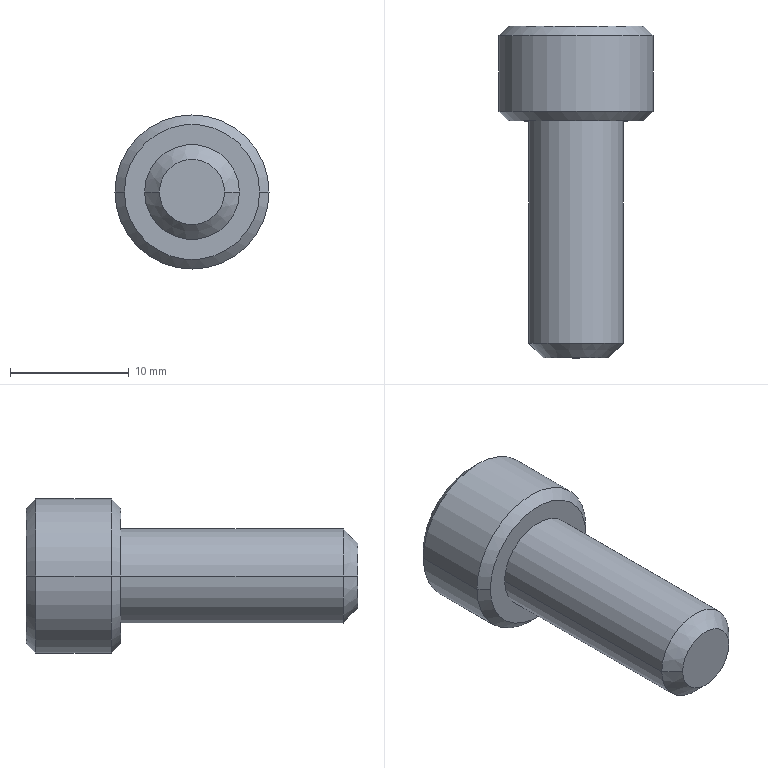Part | STEP file | BB62-M8-20L-1 | 1 solid | 27 faces | box 13 x 28 x 13 mm | volume 1878 mm3 | plane 15 | cone 8 | cylinder 4 | commonest cylinder face diameters 8 x2 13 x2
STEP:
#1=CARTESIAN_POINT('',(0.,2.02,0.));
#2=VERTEX_POINT('',#1);
#3=CARTESIAN_POINT('',(3.43,4.,0.));
#4=VERTEX_POINT('',#3);
#5=CARTESIAN_POINT('',(0.,2.02,0.));
#6=DIRECTION('',(0.866,0.5,0.));
#7=VECTOR('',#6,1000.);
#8=LINE('',#5,#7);
#9=EDGE_CURVE('',#2,#4,#8,.T.);
#10=ORIENTED_EDGE('',*,*,#9,.F.);
#11=CARTESIAN_POINT('',(-3.43,4.,0.));
#12=VERTEX_POINT('',#11);
#13=CARTESIAN_POINT('',(0.,2.02,0.));
#14=DIRECTION('',(-0.866,0.5,0.));
#15=VECTOR('',#14,1000.);
#16=LINE('',#13,#15);
#17=EDGE_CURVE('',#2,#12,#16,.T.);
#18=ORIENTED_EDGE('',*,*,#17,.T.);
#19=CARTESIAN_POINT('',(-2.97,4.,1.715));
#20=VERTEX_POINT('',#19);
#21=CARTESIAN_POINT('',(0.,4.,0.));
#22=DIRECTION('',(0.,-1.,0.));
#23=DIRECTION('',(-1.,0.,0.));
#24=AXIS2_PLACEMENT_3D('',#21,#22,#23);
#25=CIRCLE('',#24,3.43);
#26=EDGE_CURVE('',#20,#12,#25,.T.);
#27=ORIENTED_EDGE('',*,*,#26,.F.);
#28=CARTESIAN_POINT('',(0.,4.,3.43));
#29=VERTEX_POINT('',#28);
#30=CARTESIAN_POINT('',(0.,4.,0.));
#31=DIRECTION('',(0.,-1.,0.));
#32=DIRECTION('',(-1.,0.,0.));
#33=AXIS2_PLACEMENT_3D('',#30,#31,#32);
#34=CIRCLE('',#33,3.43);
#35=EDGE_CURVE('',#29,#20,#34,.T.);
#36=ORIENTED_EDGE('',*,*,#35,.F.);
#37=CARTESIAN_POINT('',(2.97,4.,1.715));
#38=VERTEX_POINT('',#37);
#39=CARTESIAN_POINT('',(0.,4.,0.));
#40=DIRECTION('',(0.,-1.,0.));
#41=DIRECTION('',(-1.,0.,0.));
#42=AXIS2_PLACEMENT_3D('',#39,#40,#41);
#43=CIRCLE('',#42,3.43);
#44=EDGE_CURVE('',#38,#29,#43,.T.);
#45=ORIENTED_EDGE('',*,*,#44,.F.);
#46=CARTESIAN_POINT('',(0.,4.,0.));
#47=DIRECTION('',(0.,-1.,0.));
#48=DIRECTION('',(-1.,0.,0.));
#49=AXIS2_PLACEMENT_3D('',#46,#47,#48);
#50=CIRCLE('',#49,3.43);
#51=EDGE_CURVE('',#4,#38,#50,.T.);
#52=ORIENTED_EDGE('',*,*,#51,.F.);
#53=EDGE_LOOP('',(#10,#18,#27,#36,#45,#52));
#54=FACE_OUTER_BOUND('',#53,.T.);
#55=CARTESIAN_POINT('',(0.,1002.02,0.));
#56=DIRECTION('',(0.,1.,0.));
#57=DIRECTION('',(1.,0.,0.));
#58=AXIS2_PLACEMENT_3D('',#55,#56,#57);
#59=CONICAL_SURFACE('',#58,1732.051,1.047);
#60=ADVANCED_FACE('',(#54),#59,.F.);
#61=CARTESIAN_POINT('',(2.75,-20.,0.));
#62=VERTEX_POINT('',#61);
#63=CARTESIAN_POINT('',(-2.75,-20.,0.));
#64=VERTEX_POINT('',#63);
#65=CARTESIAN_POINT('',(0.,-20.,0.));
#66=DIRECTION('',(0.,1.,0.));
#67=DIRECTION('',(1.,0.,0.));
#68=AXIS2_PLACEMENT_3D('',#65,#66,#67);
#69=CIRCLE('',#68,2.75);
#70=EDGE_CURVE('',#62,#64,#69,.T.);
#71=ORIENTED_EDGE('',*,*,#70,.T.);
#72=CARTESIAN_POINT('',(-4.,-18.75,0.));
#73=VERTEX_POINT('',#72);
#74=CARTESIAN_POINT('',(-2.75,-20.,0.));
#75=DIRECTION('',(-0.7071,0.7071,0.));
#76=VECTOR('',#75,1000.);
#77=LINE('',#74,#76);
#78=EDGE_CURVE('',#64,#73,#77,.T.);
#79=ORIENTED_EDGE('',*,*,#78,.T.);
#80=CARTESIAN_POINT('',(4.,-18.75,0.));
#81=VERTEX_POINT('',#80);
#82=CARTESIAN_POINT('',(0.,-18.75,0.));
#83=DIRECTION('',(0.,-1.,0.));
#84=DIRECTION('',(-1.,0.,0.));
#85=AXIS2_PLACEMENT_3D('',#82,#83,#84);
#86=CIRCLE('',#85,4.);
#87=EDGE_CURVE('',#73,#81,#86,.T.);
#88=ORIENTED_EDGE('',*,*,#87,.T.);
#89=CARTESIAN_POINT('',(2.75,-20.,0.));
#90=DIRECTION('',(0.7071,0.7071,0.));
#91=VECTOR('',#90,1000.);
#92=LINE('',#89,#91);
#93=EDGE_CURVE('',#62,#81,#92,.T.);
#94=ORIENTED_EDGE('',*,*,#93,.F.);
#95=EDGE_LOOP('',(#71,#79,#88,#94));
#96=FACE_OUTER_BOUND('',#95,.T.);
#97=CARTESIAN_POINT('',(0.,-20.,0.));
#98=DIRECTION('',(0.,1.,0.));
#99=DIRECTION('',(1.,0.,0.));
#100=AXIS2_PLACEMENT_3D('',#97,#98,#99);
#101=CONICAL_SURFACE('',#100,2.75,0.7854);
#102=ADVANCED_FACE('',(#96),#101,.T.);
#103=ORIENTED_EDGE('',*,*,#87,.F.);
#104=CARTESIAN_POINT('',(-4.,0.,0.));
#105=VERTEX_POINT('',#104);
#106=CARTESIAN_POINT('',(-4.,-18.75,0.));
#107=DIRECTION('',(0.,1.,0.));
#108=VECTOR('',#107,1000.);
#109=LINE('',#106,#108);
#110=EDGE_CURVE('',#73,#105,#109,.T.);
#111=ORIENTED_EDGE('',*,*,#110,.T.);
#112=CARTESIAN_POINT('',(4.,0.,0.));
#113=VERTEX_POINT('',#112);
#114=CARTESIAN_POINT('',(0.,0.,0.));
#115=DIRECTION('',(0.,-1.,0.));
#116=DIRECTION('',(-1.,0.,0.));
#117=AXIS2_PLACEMENT_3D('',#114,#115,#116);
#118=CIRCLE('',#117,4.);
#119=EDGE_CURVE('',#105,#113,#118,.T.);
#120=ORIENTED_EDGE('',*,*,#119,.T.);
#121=CARTESIAN_POINT('',(4.,-18.75,0.));
#122=DIRECTION('',(0.,1.,0.));
#123=VECTOR('',#122,1000.);
#124=LINE('',#121,#123);
#125=EDGE_CURVE('',#81,#113,#124,.T.);
#126=ORIENTED_EDGE('',*,*,#125,.F.);
#127=EDGE_LOOP('',(#103,#111,#120,#126));
#128=FACE_OUTER_BOUND('',#127,.T.);
#129=CARTESIAN_POINT('',(0.,-18.75,0.));
#130=DIRECTION('',(0.,1.,0.));
#131=DIRECTION('',(1.,0.,0.));
#132=AXIS2_PLACEMENT_3D('',#129,#130,#131);
#133=CYLINDRICAL_SURFACE('',#132,4.);
#134=ADVANCED_FACE('',(#128),#133,.T.);
#135=CARTESIAN_POINT('',(-5.7,8.,0.));
#136=VERTEX_POINT('',#135);
#137=CARTESIAN_POINT('',(5.7,8.,0.));
#138=VERTEX_POINT('',#137);
#139=CARTESIAN_POINT('',(0.,8.,0.));
#140=DIRECTION('',(0.,-1.,0.));
#141=DIRECTION('',(-1.,0.,0.));
#142=AXIS2_PLACEMENT_3D('',#139,#140,#141);
#143=CIRCLE('',#142,5.7);
#144=EDGE_CURVE('',#136,#138,#143,.T.);
#145=ORIENTED_EDGE('',*,*,#144,.T.);
#146=CARTESIAN_POINT('',(6.5,7.2,0.));
#147=VERTEX_POINT('',#146);
#148=CARTESIAN_POINT('',(6.5,7.2,0.));
#149=DIRECTION('',(0.7071,-0.7071,0.));
#150=VECTOR('',#149,1000.);
#151=LINE('',#148,#150);
#152=EDGE_CURVE('',#138,#147,#151,.T.);
#153=ORIENTED_EDGE('',*,*,#152,.T.);
#154=CARTESIAN_POINT('',(-6.5,7.2,0.));
#155=VERTEX_POINT('',#154);
#156=CARTESIAN_POINT('',(0.,7.2,0.));
#157=DIRECTION('',(0.,-1.,0.));
#158=DIRECTION('',(-1.,0.,0.));
#159=AXIS2_PLACEMENT_3D('',#156,#157,#158);
#160=CIRCLE('',#159,6.5);
#161=EDGE_CURVE('',#155,#147,#160,.T.);
#162=ORIENTED_EDGE('',*,*,#161,.F.);
#163=CARTESIAN_POINT('',(-6.5,7.2,0.));
#164=DIRECTION('',(-0.7071,-0.7071,0.));
#165=VECTOR('',#164,1000.);
#166=LINE('',#163,#165);
#167=EDGE_CURVE('',#136,#155,#166,.T.);
#168=ORIENTED_EDGE('',*,*,#167,.F.);
#169=EDGE_LOOP('',(#145,#153,#162,#168));
#170=FACE_OUTER_BOUND('',#169,.T.);
#171=CARTESIAN_POINT('',(0.,7.2,0.));
#172=DIRECTION('',(0.,-1.,0.));
#173=DIRECTION('',(-1.,0.,0.));
#174=AXIS2_PLACEMENT_3D('',#171,#172,#173);
#175=CONICAL_SURFACE('',#174,6.5,0.7854);
#176=ADVANCED_FACE('',(#170),#175,.T.);
#177=ORIENTED_EDGE('',*,*,#161,.T.);
#178=CARTESIAN_POINT('',(6.5,0.8,0.));
#179=VERTEX_POINT('',#178);
#180=CARTESIAN_POINT('',(6.5,1.62,0.));
#181=DIRECTION('',(0.,-1.,0.));
#182=VECTOR('',#181,1000.);
#183=LINE('',#180,#182);
#184=EDGE_CURVE('',#147,#179,#183,.T.);
#185=ORIENTED_EDGE('',*,*,#184,.T.);
#186=CARTESIAN_POINT('',(-6.5,0.8,0.));
#187=VERTEX_POINT('',#186);
#188=CARTESIAN_POINT('',(0.,0.8,0.));
#189=DIRECTION('',(0.,-1.,0.));
#190=DIRECTION('',(-1.,0.,0.));
#191=AXIS2_PLACEMENT_3D('',#188,#189,#190);
#192=CIRCLE('',#191,6.5);
#193=EDGE_CURVE('',#187,#179,#192,.T.);
#194=ORIENTED_EDGE('',*,*,#193,.F.);
#195=CARTESIAN_POINT('',(-6.5,1.62,0.));
#196=DIRECTION('',(0.,-1.,0.));
#197=VECTOR('',#196,1000.);
#198=LINE('',#195,#197);
#199=EDGE_CURVE('',#155,#187,#198,.T.);
#200=ORIENTED_EDGE('',*,*,#199,.F.);
#201=EDGE_LOOP('',(#177,#185,#194,#200));
#202=FACE_OUTER_BOUND('',#201,.T.);
#203=CARTESIAN_POINT('',(0.,1.62,0.));
#204=DIRECTION('',(0.,-1.,0.));
#205=DIRECTION('',(-1.,0.,0.));
#206=AXIS2_PLACEMENT_3D('',#203,#204,#205);
#207=CYLINDRICAL_SURFACE('',#206,6.5);
#208=ADVANCED_FACE('',(#202),#207,.T.);
#209=CARTESIAN_POINT('',(-5.7,0.,0.));
#210=VERTEX_POINT('',#209);
#211=CARTESIAN_POINT('',(5.7,0.,0.));
#212=VERTEX_POINT('',#211);
#213=CARTESIAN_POINT('',(0.,0.,0.));
#214=DIRECTION('',(0.,-1.,0.));
#215=DIRECTION('',(-1.,0.,0.));
#216=AXIS2_PLACEMENT_3D('',#213,#214,#215);
#217=CIRCLE('',#216,5.7);
#218=EDGE_CURVE('',#210,#212,#217,.T.);
#219=ORIENTED_EDGE('',*,*,#218,.F.);
#220=CARTESIAN_POINT('',(-5.7,0.,0.));
#221=DIRECTION('',(-0.7071,0.7071,0.));
#222=VECTOR('',#221,1000.);
#223=LINE('',#220,#222);
#224=EDGE_CURVE('',#210,#187,#223,.T.);
#225=ORIENTED_EDGE('',*,*,#224,.T.);
#226=ORIENTED_EDGE('',*,*,#193,.T.);
#227=CARTESIAN_POINT('',(5.7,0.,0.));
#228=DIRECTION('',(0.7071,0.7071,0.));
#229=VECTOR('',#228,1000.);
#230=LINE('',#227,#229);
#231=EDGE_CURVE('',#212,#179,#230,.T.);
#232=ORIENTED_EDGE('',*,*,#231,.F.);
#233=EDGE_LOOP('',(#219,#225,#226,#232));
#234=FACE_OUTER_BOUND('',#233,.T.);
#235=CARTESIAN_POINT('',(0.,0.,0.));
#236=DIRECTION('',(0.,1.,0.));
#237=DIRECTION('',(1.,0.,0.));
#238=AXIS2_PLACEMENT_3D('',#235,#236,#237);
#239=CONICAL_SURFACE('',#238,5.7,0.7854);
#240=ADVANCED_FACE('',(#234),#239,.T.);
#241=ORIENTED_EDGE('',*,*,#144,.F.);
#242=CARTESIAN_POINT('',(0.,8.,0.));
#243=DIRECTION('',(0.,-1.,0.));
#244=DIRECTION('',(-1.,0.,0.));
#245=AXIS2_PLACEMENT_3D('',#242,#243,#244);
#246=CIRCLE('',#245,5.7);
#247=EDGE_CURVE('',#138,#136,#246,.T.);
#248=ORIENTED_EDGE('',*,*,#247,.F.);
#249=EDGE_LOOP('',(#241,#248));
#250=FACE_OUTER_BOUND('',#249,.T.);
#251=CARTESIAN_POINT('',(0.,8.,-3.43));
#252=VERTEX_POINT('',#251);
#253=CARTESIAN_POINT('',(-2.97,8.,-1.715));
#254=VERTEX_POINT('',#253);
#255=CARTESIAN_POINT('',(0.,8.,-3.43));
#256=DIRECTION('',(-0.866,0.,0.5));
#257=VECTOR('',#256,1000.);
#258=LINE('',#255,#257);
#259=EDGE_CURVE('',#252,#254,#258,.T.);
#260=ORIENTED_EDGE('',*,*,#259,.F.);
#261=CARTESIAN_POINT('',(2.97,8.,-1.715));
#262=VERTEX_POINT('',#261);
#263=CARTESIAN_POINT('',(2.97,8.,-1.715));
#264=DIRECTION('',(-0.866,0.,-0.5));
#265=VECTOR('',#264,1000.);
#266=LINE('',#263,#265);
#267=EDGE_CURVE('',#262,#252,#266,.T.);
#268=ORIENTED_EDGE('',*,*,#267,.F.);
#269=CARTESIAN_POINT('',(2.97,8.,1.715));
#270=VERTEX_POINT('',#269);
#271=CARTESIAN_POINT('',(2.97,8.,1.715));
#272=DIRECTION('',(0.,0.,-1.));
#273=VECTOR('',#272,1000.);
#274=LINE('',#271,#273);
#275=EDGE_CURVE('',#270,#262,#274,.T.);
#276=ORIENTED_EDGE('',*,*,#275,.F.);
#277=CARTESIAN_POINT('',(0.,8.,3.43));
#278=VERTEX_POINT('',#277);
#279=CARTESIAN_POINT('',(0.,8.,3.43));
#280=DIRECTION('',(0.866,0.,-0.5));
#281=VECTOR('',#280,1000.);
#282=LINE('',#279,#281);
#283=EDGE_CURVE('',#278,#270,#282,.T.);
#284=ORIENTED_EDGE('',*,*,#283,.F.);
#285=CARTESIAN_POINT('',(-2.97,8.,1.715));
#286=VERTEX_POINT('',#285);
#287=CARTESIAN_POINT('',(-2.97,8.,1.715));
#288=DIRECTION('',(0.866,0.,0.5));
#289=VECTOR('',#288,1000.);
#290=LINE('',#287,#289);
#291=EDGE_CURVE('',#286,#278,#290,.T.);
#292=ORIENTED_EDGE('',*,*,#291,.F.);
#293=CARTESIAN_POINT('',(-2.97,8.,-1.715));
#294=DIRECTION('',(0.,0.,1.));
#295=VECTOR('',#294,1000.);
#296=LINE('',#293,#295);
#297=EDGE_CURVE('',#254,#286,#296,.T.);
#298=ORIENTED_EDGE('',*,*,#297,.F.);
#299=EDGE_LOOP('',(#260,#268,#276,#284,#292,#298));
#300=FACE_BOUND('',#299,.T.);
#301=CARTESIAN_POINT('',(5.7,8.,0.));
#302=DIRECTION('',(0.,1.,0.));
#303=DIRECTION('',(1.,0.,0.));
#304=AXIS2_PLACEMENT_3D('',#301,#302,#303);
#305=PLANE('',#304);
#306=ADVANCED_FACE('',(#250,#300),#305,.T.);
#307=CARTESIAN_POINT('',(0.,0.,0.));
#308=DIRECTION('',(0.,-1.,0.));
#309=DIRECTION('',(-1.,0.,0.));
#310=AXIS2_PLACEMENT_3D('',#307,#308,#309);
#311=CIRCLE('',#310,4.);
#312=EDGE_CURVE('',#113,#105,#311,.T.);
#313=ORIENTED_EDGE('',*,*,#312,.F.);
#314=ORIENTED_EDGE('',*,*,#119,.F.);
#315=EDGE_LOOP('',(#313,#314));
#316=FACE_BOUND('',#315,.T.);
#317=CARTESIAN_POINT('',(0.,0.,0.));
#318=DIRECTION('',(0.,-1.,0.));
#319=DIRECTION('',(-1.,0.,0.));
#320=AXIS2_PLACEMENT_3D('',#317,#318,#319);
#321=CIRCLE('',#320,5.7);
#322=EDGE_CURVE('',#212,#210,#321,.T.);
#323=ORIENTED_EDGE('',*,*,#322,.T.);
#324=ORIENTED_EDGE('',*,*,#218,.T.);
#325=EDGE_LOOP('',(#323,#324));
#326=FACE_OUTER_BOUND('',#325,.T.);
#327=CARTESIAN_POINT('',(0.,0.,0.));
#328=DIRECTION('',(0.,-1.,0.));
#329=DIRECTION('',(-1.,0.,0.));
#330=AXIS2_PLACEMENT_3D('',#327,#328,#329);
#331=PLANE('',#330);
#332=ADVANCED_FACE('',(#316,#326),#331,.T.);
#333=ORIENTED_EDGE('',*,*,#224,.F.);
#334=ORIENTED_EDGE('',*,*,#322,.F.);
#335=ORIENTED_EDGE('',*,*,#231,.T.);
#336=CARTESIAN_POINT('',(0.,0.8,0.));
#337=DIRECTION('',(0.,-1.,0.));
#338=DIRECTION('',(-1.,0.,0.));
#339=AXIS2_PLACEMENT_3D('',#336,#337,#338);
#340=CIRCLE('',#339,6.5);
#341=EDGE_CURVE('',#179,#187,#340,.T.);
#342=ORIENTED_EDGE('',*,*,#341,.T.);
#343=EDGE_LOOP('',(#333,#334,#335,#342));
#344=FACE_OUTER_BOUND('',#343,.T.);
#345=CARTESIAN_POINT('',(0.,0.,0.));
#346=DIRECTION('',(0.,1.,0.));
#347=DIRECTION('',(1.,0.,0.));
#348=AXIS2_PLACEMENT_3D('',#345,#346,#347);
#349=CONICAL_SURFACE('',#348,5.7,0.7854);
#350=ADVANCED_FACE('',(#344),#349,.T.);
#351=ORIENTED_EDGE('',*,*,#184,.F.);
#352=CARTESIAN_POINT('',(0.,7.2,0.));
#353=DIRECTION('',(0.,-1.,0.));
#354=DIRECTION('',(-1.,0.,0.));
#355=AXIS2_PLACEMENT_3D('',#352,#353,#354);
#356=CIRCLE('',#355,6.5);
#357=EDGE_CURVE('',#147,#155,#356,.T.);
#358=ORIENTED_EDGE('',*,*,#357,.T.);
#359=ORIENTED_EDGE('',*,*,#199,.T.);
#360=ORIENTED_EDGE('',*,*,#341,.F.);
#361=EDGE_LOOP('',(#351,#358,#359,#360));
#362=FACE_OUTER_BOUND('',#361,.T.);
#363=CARTESIAN_POINT('',(0.,1.62,0.));
#364=DIRECTION('',(0.,-1.,0.));
#365=DIRECTION('',(-1.,0.,0.));
#366=AXIS2_PLACEMENT_3D('',#363,#364,#365);
#367=CYLINDRICAL_SURFACE('',#366,6.5);
#368=ADVANCED_FACE('',(#362),#367,.T.);
#369=ORIENTED_EDGE('',*,*,#152,.F.);
#370=ORIENTED_EDGE('',*,*,#247,.T.);
#371=ORIENTED_EDGE('',*,*,#167,.T.);
#372=ORIENTED_EDGE('',*,*,#357,.F.);
#373=EDGE_LOOP('',(#369,#370,#371,#372));
#374=FACE_OUTER_BOUND('',#373,.T.);
#375=CARTESIAN_POINT('',(0.,7.2,0.));
#376=DIRECTION('',(0.,-1.,0.));
#377=DIRECTION('',(-1.,0.,0.));
#378=AXIS2_PLACEMENT_3D('',#375,#376,#377);
#379=CONICAL_SURFACE('',#378,6.5,0.7854);
#380=ADVANCED_FACE('',(#374),#379,.T.);
#381=ORIENTED_EDGE('',*,*,#110,.F.);
#382=CARTESIAN_POINT('',(0.,-18.75,0.));
#383=DIRECTION('',(0.,-1.,0.));
#384=DIRECTION('',(-1.,0.,0.));
#385=AXIS2_PLACEMENT_3D('',#382,#383,#384);
#386=CIRCLE('',#385,4.);
#387=EDGE_CURVE('',#81,#73,#386,.T.);
#388=ORIENTED_EDGE('',*,*,#387,.F.);
#389=ORIENTED_EDGE('',*,*,#125,.T.);
#390=ORIENTED_EDGE('',*,*,#312,.T.);
#391=EDGE_LOOP('',(#381,#388,#389,#390));
#392=FACE_OUTER_BOUND('',#391,.T.);
#393=CARTESIAN_POINT('',(0.,-18.75,0.));
#394=DIRECTION('',(0.,1.,0.));
#395=DIRECTION('',(1.,0.,0.));
#396=AXIS2_PLACEMENT_3D('',#393,#394,#395);
#397=CYLINDRICAL_SURFACE('',#396,4.);
#398=ADVANCED_FACE('',(#392),#397,.T.);
#399=ORIENTED_EDGE('',*,*,#70,.F.);
#400=CARTESIAN_POINT('',(0.,-20.,0.));
#401=DIRECTION('',(0.,1.,0.));
#402=DIRECTION('',(1.,0.,0.));
#403=AXIS2_PLACEMENT_3D('',#400,#401,#402);
#404=CIRCLE('',#403,2.75);
#405=EDGE_CURVE('',#64,#62,#404,.T.);
#406=ORIENTED_EDGE('',*,*,#405,.F.);
#407=EDGE_LOOP('',(#399,#406));
#408=FACE_OUTER_BOUND('',#407,.T.);
#409=CARTESIAN_POINT('',(0.,-20.,0.));
#410=DIRECTION('',(0.,-1.,0.));
#411=DIRECTION('',(-1.,0.,0.));
#412=AXIS2_PLACEMENT_3D('',#409,#410,#411);
#413=PLANE('',#412);
#414=ADVANCED_FACE('',(#408),#413,.T.);
#415=ORIENTED_EDGE('',*,*,#78,.F.);
#416=ORIENTED_EDGE('',*,*,#405,.T.);
#417=ORIENTED_EDGE('',*,*,#93,.T.);
#418=ORIENTED_EDGE('',*,*,#387,.T.);
#419=EDGE_LOOP('',(#415,#416,#417,#418));
#420=FACE_OUTER_BOUND('',#419,.T.);
#421=CARTESIAN_POINT('',(0.,-20.,0.));
#422=DIRECTION('',(0.,1.,0.));
#423=DIRECTION('',(1.,0.,0.));
#424=AXIS2_PLACEMENT_3D('',#421,#422,#423);
#425=CONICAL_SURFACE('',#424,2.75,0.7854);
#426=ADVANCED_FACE('',(#420),#425,.T.);
#427=CARTESIAN_POINT('',(2.97,4.,-1.715));
#428=VERTEX_POINT('',#427);
#429=CARTESIAN_POINT('',(0.,4.,-3.43));
#430=VERTEX_POINT('',#429);
#431=CARTESIAN_POINT('',(2.97,4.,-1.715));
#432=DIRECTION('',(-0.866,0.,-0.5));
#433=VECTOR('',#432,1000.);
#434=LINE('',#431,#433);
#435=EDGE_CURVE('',#428,#430,#434,.T.);
#436=ORIENTED_EDGE('',*,*,#435,.F.);
#437=CARTESIAN_POINT('',(2.97,8.,-1.715));
#438=DIRECTION('',(0.,-1.,0.));
#439=VECTOR('',#438,1000.);
#440=LINE('',#437,#439);
#441=EDGE_CURVE('',#262,#428,#440,.T.);
#442=ORIENTED_EDGE('',*,*,#441,.F.);
#443=ORIENTED_EDGE('',*,*,#267,.T.);
#444=CARTESIAN_POINT('',(0.,8.,-3.43));
#445=DIRECTION('',(0.,-1.,0.));
#446=VECTOR('',#445,1000.);
#447=LINE('',#444,#446);
#448=EDGE_CURVE('',#252,#430,#447,.T.);
#449=ORIENTED_EDGE('',*,*,#448,.T.);
#450=EDGE_LOOP('',(#436,#442,#443,#449));
#451=FACE_OUTER_BOUND('',#450,.T.);
#452=CARTESIAN_POINT('',(2.97,8.,-1.715));
#453=DIRECTION('',(-0.5,0.,0.866));
#454=DIRECTION('',(0.866,0.,0.5));
#455=AXIS2_PLACEMENT_3D('',#452,#453,#454);
#456=PLANE('',#455);
#457=ADVANCED_FACE('',(#451),#456,.T.);
#458=CARTESIAN_POINT('',(-2.97,4.,-1.715));
#459=VERTEX_POINT('',#458);
#460=CARTESIAN_POINT('',(0.,4.,-3.43));
#461=DIRECTION('',(-0.866,0.,0.5));
#462=VECTOR('',#461,1000.);
#463=LINE('',#460,#462);
#464=EDGE_CURVE('',#430,#459,#463,.T.);
#465=ORIENTED_EDGE('',*,*,#464,.F.);
#466=ORIENTED_EDGE('',*,*,#448,.F.);
#467=ORIENTED_EDGE('',*,*,#259,.T.);
#468=CARTESIAN_POINT('',(-2.97,8.,-1.715));
#469=DIRECTION('',(0.,-1.,0.));
#470=VECTOR('',#469,1000.);
#471=LINE('',#468,#470);
#472=EDGE_CURVE('',#254,#459,#471,.T.);
#473=ORIENTED_EDGE('',*,*,#472,.T.);
#474=EDGE_LOOP('',(#465,#466,#467,#473));
#475=FACE_OUTER_BOUND('',#474,.T.);
#476=CARTESIAN_POINT('',(0.,8.,-3.43));
#477=DIRECTION('',(0.5,0.,0.866));
#478=DIRECTION('',(0.866,0.,-0.5));
#479=AXIS2_PLACEMENT_3D('',#476,#477,#478);
#480=PLANE('',#479);
#481=ADVANCED_FACE('',(#475),#480,.T.);
#482=CARTESIAN_POINT('',(-2.97,4.,-1.715));
#483=DIRECTION('',(0.,0.,1.));
#484=VECTOR('',#483,1000.);
#485=LINE('',#482,#484);
#486=EDGE_CURVE('',#459,#20,#485,.T.);
#487=ORIENTED_EDGE('',*,*,#486,.F.);
#488=ORIENTED_EDGE('',*,*,#472,.F.);
#489=ORIENTED_EDGE('',*,*,#297,.T.);
#490=CARTESIAN_POINT('',(-2.97,8.,1.715));
#491=DIRECTION('',(0.,-1.,0.));
#492=VECTOR('',#491,1000.);
#493=LINE('',#490,#492);
#494=EDGE_CURVE('',#286,#20,#493,.T.);
#495=ORIENTED_EDGE('',*,*,#494,.T.);
#496=EDGE_LOOP('',(#487,#488,#489,#495));
#497=FACE_OUTER_BOUND('',#496,.T.);
#498=CARTESIAN_POINT('',(-2.97,8.,-1.715));
#499=DIRECTION('',(1.,0.,0.));
#500=DIRECTION('',(0.,0.,-1.));
#501=AXIS2_PLACEMENT_3D('',#498,#499,#500);
#502=PLANE('',#501);
#503=ADVANCED_FACE('',(#497),#502,.T.);
#504=CARTESIAN_POINT('',(-2.97,4.,1.715));
#505=DIRECTION('',(0.866,0.,0.5));
#506=VECTOR('',#505,1000.);
#507=LINE('',#504,#506);
#508=EDGE_CURVE('',#20,#29,#507,.T.);
#509=ORIENTED_EDGE('',*,*,#508,.F.);
#510=ORIENTED_EDGE('',*,*,#494,.F.);
#511=ORIENTED_EDGE('',*,*,#291,.T.);
#512=CARTESIAN_POINT('',(0.,8.,3.43));
#513=DIRECTION('',(0.,-1.,0.));
#514=VECTOR('',#513,1000.);
#515=LINE('',#512,#514);
#516=EDGE_CURVE('',#278,#29,#515,.T.);
#517=ORIENTED_EDGE('',*,*,#516,.T.);
#518=EDGE_LOOP('',(#509,#510,#511,#517));
#519=FACE_OUTER_BOUND('',#518,.T.);
#520=CARTESIAN_POINT('',(-2.97,8.,1.715));
#521=DIRECTION('',(0.5,0.,-0.866));
#522=DIRECTION('',(-0.866,0.,-0.5));
#523=AXIS2_PLACEMENT_3D('',#520,#521,#522);
#524=PLANE('',#523);
#525=ADVANCED_FACE('',(#519),#524,.T.);
#526=CARTESIAN_POINT('',(0.,4.,3.43));
#527=DIRECTION('',(0.866,0.,-0.5));
#528=VECTOR('',#527,1000.);
#529=LINE('',#526,#528);
#530=EDGE_CURVE('',#29,#38,#529,.T.);
#531=ORIENTED_EDGE('',*,*,#530,.F.);
#532=ORIENTED_EDGE('',*,*,#516,.F.);
#533=ORIENTED_EDGE('',*,*,#283,.T.);
#534=CARTESIAN_POINT('',(2.97,8.,1.715));
#535=DIRECTION('',(0.,-1.,0.));
#536=VECTOR('',#535,1000.);
#537=LINE('',#534,#536);
#538=EDGE_CURVE('',#270,#38,#537,.T.);
#539=ORIENTED_EDGE('',*,*,#538,.T.);
#540=EDGE_LOOP('',(#531,#532,#533,#539));
#541=FACE_OUTER_BOUND('',#540,.T.);
#542=CARTESIAN_POINT('',(0.,8.,3.43));
#543=DIRECTION('',(-0.5,0.,-0.866));
#544=DIRECTION('',(-0.866,0.,0.5));
#545=AXIS2_PLACEMENT_3D('',#542,#543,#544);
#546=PLANE('',#545);
#547=ADVANCED_FACE('',(#541),#546,.T.);
#548=CARTESIAN_POINT('',(2.97,4.,1.715));
#549=DIRECTION('',(0.,0.,-1.));
#550=VECTOR('',#549,1000.);
#551=LINE('',#548,#550);
#552=EDGE_CURVE('',#38,#428,#551,.T.);
#553=ORIENTED_EDGE('',*,*,#552,.F.);
#554=ORIENTED_EDGE('',*,*,#538,.F.);
#555=ORIENTED_EDGE('',*,*,#275,.T.);
#556=ORIENTED_EDGE('',*,*,#441,.T.);
#557=EDGE_LOOP('',(#553,#554,#555,#556));
#558=FACE_OUTER_BOUND('',#557,.T.);
#559=CARTESIAN_POINT('',(2.97,8.,1.715));
#560=DIRECTION('',(-1.,0.,0.));
#561=DIRECTION('',(0.,0.,1.));
#562=AXIS2_PLACEMENT_3D('',#559,#560,#561);
#563=PLANE('',#562);
#564=ADVANCED_FACE('',(#558),#563,.T.);
#565=ORIENTED_EDGE('',*,*,#435,.T.);
#566=CARTESIAN_POINT('',(0.,4.,0.));
#567=DIRECTION('',(0.,-1.,0.));
#568=DIRECTION('',(-1.,0.,0.));
#569=AXIS2_PLACEMENT_3D('',#566,#567,#568);
#570=CIRCLE('',#569,3.43);
#571=EDGE_CURVE('',#430,#428,#570,.T.);
#572=ORIENTED_EDGE('',*,*,#571,.T.);
#573=EDGE_LOOP('',(#565,#572));
#574=FACE_OUTER_BOUND('',#573,.T.);
#575=CARTESIAN_POINT('',(0.,4.,0.));
#576=DIRECTION('',(0.,1.,0.));
#577=DIRECTION('',(1.,0.,0.));
#578=AXIS2_PLACEMENT_3D('',#575,#576,#577);
#579=PLANE('',#578);
#580=ADVANCED_FACE('',(#574),#579,.F.);
#581=ORIENTED_EDGE('',*,*,#552,.T.);
#582=CARTESIAN_POINT('',(0.,4.,0.));
#583=DIRECTION('',(0.,-1.,0.));
#584=DIRECTION('',(-1.,0.,0.));
#585=AXIS2_PLACEMENT_3D('',#582,#583,#584);
#586=CIRCLE('',#585,3.43);
#587=EDGE_CURVE('',#428,#4,#586,.T.);
#588=ORIENTED_EDGE('',*,*,#587,.T.);
#589=ORIENTED_EDGE('',*,*,#51,.T.);
#590=EDGE_LOOP('',(#581,#588,#589));
#591=FACE_OUTER_BOUND('',#590,.T.);
#592=CARTESIAN_POINT('',(0.,4.,0.));
#593=DIRECTION('',(0.,1.,0.));
#594=DIRECTION('',(1.,0.,0.));
#595=AXIS2_PLACEMENT_3D('',#592,#593,#594);
#596=PLANE('',#595);
#597=ADVANCED_FACE('',(#591),#596,.F.);
#598=ORIENTED_EDGE('',*,*,#530,.T.);
#599=ORIENTED_EDGE('',*,*,#44,.T.);
#600=EDGE_LOOP('',(#598,#599));
#601=FACE_OUTER_BOUND('',#600,.T.);
#602=CARTESIAN_POINT('',(0.,4.,0.));
#603=DIRECTION('',(0.,1.,0.));
#604=DIRECTION('',(1.,0.,0.));
#605=AXIS2_PLACEMENT_3D('',#602,#603,#604);
#606=PLANE('',#605);
#607=ADVANCED_FACE('',(#601),#606,.F.);
#608=ORIENTED_EDGE('',*,*,#508,.T.);
#609=ORIENTED_EDGE('',*,*,#35,.T.);
#610=EDGE_LOOP('',(#608,#609));
#611=FACE_OUTER_BOUND('',#610,.T.);
#612=CARTESIAN_POINT('',(0.,4.,0.));
#613=DIRECTION('',(0.,1.,0.));
#614=DIRECTION('',(1.,0.,0.));
#615=AXIS2_PLACEMENT_3D('',#612,#613,#614);
#616=PLANE('',#615);
#617=ADVANCED_FACE('',(#611),#616,.F.);
#618=ORIENTED_EDGE('',*,*,#486,.T.);
#619=ORIENTED_EDGE('',*,*,#26,.T.);
#620=CARTESIAN_POINT('',(0.,4.,0.));
#621=DIRECTION('',(0.,-1.,0.));
#622=DIRECTION('',(-1.,0.,0.));
#623=AXIS2_PLACEMENT_3D('',#620,#621,#622);
#624=CIRCLE('',#623,3.43);
#625=EDGE_CURVE('',#12,#459,#624,.T.);
#626=ORIENTED_EDGE('',*,*,#625,.T.);
#627=EDGE_LOOP('',(#618,#619,#626));
#628=FACE_OUTER_BOUND('',#627,.T.);
#629=CARTESIAN_POINT('',(0.,4.,0.));
#630=DIRECTION('',(0.,1.,0.));
#631=DIRECTION('',(1.,0.,0.));
#632=AXIS2_PLACEMENT_3D('',#629,#630,#631);
#633=PLANE('',#632);
#634=ADVANCED_FACE('',(#628),#633,.F.);
#635=ORIENTED_EDGE('',*,*,#464,.T.);
#636=CARTESIAN_POINT('',(0.,4.,0.));
#637=DIRECTION('',(0.,-1.,0.));
#638=DIRECTION('',(-1.,0.,0.));
#639=AXIS2_PLACEMENT_3D('',#636,#637,#638);
#640=CIRCLE('',#639,3.43);
#641=EDGE_CURVE('',#459,#430,#640,.T.);
#642=ORIENTED_EDGE('',*,*,#641,.T.);
#643=EDGE_LOOP('',(#635,#642));
#644=FACE_OUTER_BOUND('',#643,.T.);
#645=CARTESIAN_POINT('',(0.,4.,0.));
#646=DIRECTION('',(0.,1.,0.));
#647=DIRECTION('',(1.,0.,0.));
#648=AXIS2_PLACEMENT_3D('',#645,#646,#647);
#649=PLANE('',#648);
#650=ADVANCED_FACE('',(#644),#649,.F.);
#651=ORIENTED_EDGE('',*,*,#17,.F.);
#652=ORIENTED_EDGE('',*,*,#9,.T.);
#653=ORIENTED_EDGE('',*,*,#587,.F.);
#654=ORIENTED_EDGE('',*,*,#571,.F.);
#655=ORIENTED_EDGE('',*,*,#641,.F.);
#656=ORIENTED_EDGE('',*,*,#625,.F.);
#657=EDGE_LOOP('',(#651,#652,#653,#654,#655,#656));
#658=FACE_OUTER_BOUND('',#657,.T.);
#659=CARTESIAN_POINT('',(0.,1002.02,0.));
#660=DIRECTION('',(0.,1.,0.));
#661=DIRECTION('',(1.,0.,0.));
#662=AXIS2_PLACEMENT_3D('',#659,#660,#661);
#663=CONICAL_SURFACE('',#662,1732.051,1.047);
#664=ADVANCED_FACE('',(#658),#663,.F.);
#665=CLOSED_SHELL('',(#60,#102,#134,#176,#208,#240,#306,#332,#350,#368,#380,#398,#414,#426,#457,#481,#503,#525,#547,#564,#580,#597,#607,#617,#634,#650,#664));
#666=MANIFOLD_SOLID_BREP('',#665);
#667=CARTESIAN_POINT('',(0.,0.,0.));
#668=DIRECTION('',(0.,0.,1.));
#669=DIRECTION('',(1.,0.,0.));
#670=AXIS2_PLACEMENT_3D('',#667,#668,#669);
#671=(LENGTH_UNIT()NAMED_UNIT(*)SI_UNIT(.MILLI.,.METRE.));
#672=UNCERTAINTY_MEASURE_WITH_UNIT(LENGTH_MEASURE(0.00001),#671,'','');
#673=(NAMED_UNIT(*)PLANE_ANGLE_UNIT()SI_UNIT($,.RADIAN.));
#674=(NAMED_UNIT(*)SI_UNIT($,.STERADIAN.)SOLID_ANGLE_UNIT());
#675=(GEOMETRIC_REPRESENTATION_CONTEXT(3)GLOBAL_UNCERTAINTY_ASSIGNED_CONTEXT((#672))GLOBAL_UNIT_ASSIGNED_CONTEXT((#671,#673,#674))REPRESENTATION_CONTEXT('',''));
#676=ADVANCED_BREP_SHAPE_REPRESENTATION('',(#666,#670),#675);